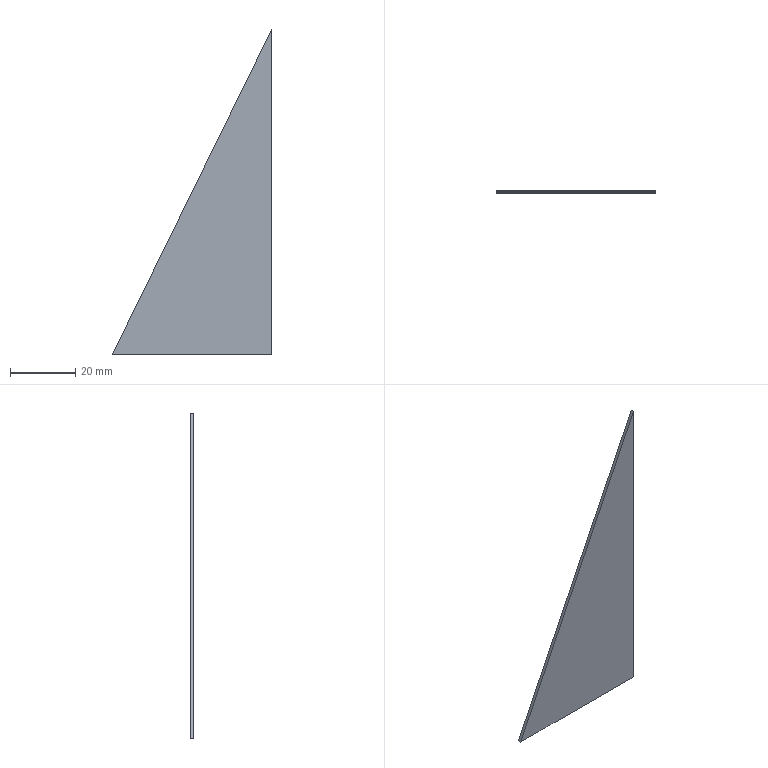Part | STEP file | RJWD-DY-0114_X2_75356C145B898_5 | 1 solid | 5 faces | box 48.998 x 1 x 99.996 mm | volume 2450 mm3 | plane 5
STEP:
#1=CARTESIAN_POINT('',(0.,0.,0.));
#2=DIRECTION('',(0.,0.,1.));
#3=DIRECTION('',(1.,0.,0.));
#4=AXIS2_PLACEMENT_3D('',#1,#2,#3);
#5=CARTESIAN_POINT('',(657.039,5199.7,119.644));
#6=VERTEX_POINT('',#5);
#7=CARTESIAN_POINT('',(657.039,5199.7,219.64));
#8=VERTEX_POINT('',#7);
#9=CARTESIAN_POINT('',(657.039,5199.7,119.644));
#10=DIRECTION('',(0.,0.,1.));
#11=VECTOR('',#10,1.);
#12=LINE('',#9,#11);
#13=CARTESIAN_POINT('',(608.041,5199.7,219.644));
#14=DIRECTION('',(0.,1.,0.));
#15=DIRECTION('',(0.,0.,1.));
#16=AXIS2_PLACEMENT_3D('',#13,#14,#15);
#17=PLANE('',#16);
#18=CARTESIAN_POINT('',(-100.,48.998));
#19=DIRECTION('',(1.,0.));
#20=VECTOR('',#19,1.);
#21=LINE('',#18,#20);
#22=(GEOMETRIC_REPRESENTATION_CONTEXT(2)PARAMETRIC_REPRESENTATION_CONTEXT()REPRESENTATION_CONTEXT('',''));
#23=DEFINITIONAL_REPRESENTATION('',(#21),#22);
#24=PCURVE('',#17,#23);
#25=CARTESIAN_POINT('',(657.039,5199.7,219.644));
#26=DIRECTION('',(-1.,0.,0.));
#27=DIRECTION('',(0.,0.,1.));
#28=AXIS2_PLACEMENT_3D('',#25,#26,#27);
#29=PLANE('',#28);
#30=CARTESIAN_POINT('',(-100.,0.));
#31=DIRECTION('',(1.,0.));
#32=VECTOR('',#31,1.);
#33=LINE('',#30,#32);
#34=(GEOMETRIC_REPRESENTATION_CONTEXT(2)PARAMETRIC_REPRESENTATION_CONTEXT()REPRESENTATION_CONTEXT('',''));
#35=DEFINITIONAL_REPRESENTATION('',(#33),#34);
#36=PCURVE('',#29,#35);
#37=SURFACE_CURVE('',#12,(#24,#36),.PCURVE_S1.);
#38=EDGE_CURVE('',#6,#8,#37,.T.);
#39=ORIENTED_EDGE('',*,*,#38,.F.);
#40=CARTESIAN_POINT('',(608.041,5199.7,119.644));
#41=VERTEX_POINT('',#40);
#42=CARTESIAN_POINT('',(657.039,5199.7,119.644));
#43=DIRECTION('',(-1.,0.,0.));
#44=VECTOR('',#43,1.);
#45=LINE('',#42,#44);
#46=CARTESIAN_POINT('',(-100.,48.998));
#47=DIRECTION('',(0.,-1.));
#48=VECTOR('',#47,1.);
#49=LINE('',#46,#48);
#50=(GEOMETRIC_REPRESENTATION_CONTEXT(2)PARAMETRIC_REPRESENTATION_CONTEXT()REPRESENTATION_CONTEXT('',''));
#51=DEFINITIONAL_REPRESENTATION('',(#49),#50);
#52=PCURVE('',#17,#51);
#53=CARTESIAN_POINT('',(0.,140.,119.644));
#54=DIRECTION('',(0.,0.,1.));
#55=DIRECTION('',(1.,0.,0.));
#56=AXIS2_PLACEMENT_3D('',#53,#54,#55);
#57=PLANE('',#56);
#58=CARTESIAN_POINT('',(657.039,5059.7));
#59=DIRECTION('',(-1.,0.));
#60=VECTOR('',#59,1.);
#61=LINE('',#58,#60);
#62=(GEOMETRIC_REPRESENTATION_CONTEXT(2)PARAMETRIC_REPRESENTATION_CONTEXT()REPRESENTATION_CONTEXT('',''));
#63=DEFINITIONAL_REPRESENTATION('',(#61),#62);
#64=PCURVE('',#57,#63);
#65=SURFACE_CURVE('',#45,(#52,#64),.PCURVE_S1.);
#66=EDGE_CURVE('',#6,#41,#65,.T.);
#67=ORIENTED_EDGE('',*,*,#66,.T.);
#68=CARTESIAN_POINT('',(657.039,5199.7,219.64));
#69=DIRECTION('',(-0.44,0.,-0.898));
#70=VECTOR('',#69,1.);
#71=LINE('',#68,#70);
#72=CARTESIAN_POINT('',(-0.004082,48.998));
#73=DIRECTION('',(-0.898,-0.44));
#74=VECTOR('',#73,1.);
#75=LINE('',#72,#74);
#76=(GEOMETRIC_REPRESENTATION_CONTEXT(2)PARAMETRIC_REPRESENTATION_CONTEXT()REPRESENTATION_CONTEXT('',''));
#77=DEFINITIONAL_REPRESENTATION('',(#75),#76);
#78=PCURVE('',#17,#77);
#79=CARTESIAN_POINT('',(657.041,140.,219.644));
#80=DIRECTION('',(-0.898,0.,0.44));
#81=DIRECTION('',(0.,1.,0.));
#82=AXIS2_PLACEMENT_3D('',#79,#80,#81);
#83=PLANE('',#82);
#84=CARTESIAN_POINT('',(5059.7,0.004545));
#85=DIRECTION('',(0.,1.));
#86=VECTOR('',#85,1.);
#87=LINE('',#84,#86);
#88=(GEOMETRIC_REPRESENTATION_CONTEXT(2)PARAMETRIC_REPRESENTATION_CONTEXT()REPRESENTATION_CONTEXT('',''));
#89=DEFINITIONAL_REPRESENTATION('',(#87),#88);
#90=PCURVE('',#83,#89);
#91=SURFACE_CURVE('',#71,(#78,#90),.PCURVE_S1.);
#92=EDGE_CURVE('',#8,#41,#91,.T.);
#93=ORIENTED_EDGE('',*,*,#92,.F.);
#94=EDGE_LOOP('',(#39,#67,#93));
#95=FACE_BOUND('',#94,.F.);
#96=ADVANCED_FACE('',(#95),#17,.F.);
#97=CARTESIAN_POINT('',(657.039,5200.7,119.644));
#98=VERTEX_POINT('',#97);
#99=CARTESIAN_POINT('',(657.039,5200.7,219.64));
#100=VERTEX_POINT('',#99);
#101=CARTESIAN_POINT('',(657.039,5200.7,119.644));
#102=DIRECTION('',(0.,0.,1.));
#103=VECTOR('',#102,1.);
#104=LINE('',#101,#103);
#105=CARTESIAN_POINT('',(-100.,1.));
#106=DIRECTION('',(1.,0.));
#107=VECTOR('',#106,1.);
#108=LINE('',#105,#107);
#109=(GEOMETRIC_REPRESENTATION_CONTEXT(2)PARAMETRIC_REPRESENTATION_CONTEXT()REPRESENTATION_CONTEXT('',''));
#110=DEFINITIONAL_REPRESENTATION('',(#108),#109);
#111=PCURVE('',#29,#110);
#112=CARTESIAN_POINT('',(657.039,5200.7,219.644));
#113=DIRECTION('',(0.,-1.,0.));
#114=DIRECTION('',(0.,0.,-1.));
#115=AXIS2_PLACEMENT_3D('',#112,#113,#114);
#116=PLANE('',#115);
#117=CARTESIAN_POINT('',(100.,0.));
#118=DIRECTION('',(-1.,0.));
#119=VECTOR('',#118,1.);
#120=LINE('',#117,#119);
#121=(GEOMETRIC_REPRESENTATION_CONTEXT(2)PARAMETRIC_REPRESENTATION_CONTEXT()REPRESENTATION_CONTEXT('',''));
#122=DEFINITIONAL_REPRESENTATION('',(#120),#121);
#123=PCURVE('',#116,#122);
#124=SURFACE_CURVE('',#104,(#111,#123),.PCURVE_S1.);
#125=EDGE_CURVE('',#98,#100,#124,.T.);
#126=ORIENTED_EDGE('',*,*,#125,.F.);
#127=CARTESIAN_POINT('',(657.039,5200.7,119.644));
#128=DIRECTION('',(0.,-1.,0.));
#129=VECTOR('',#128,1.);
#130=LINE('',#127,#129);
#131=CARTESIAN_POINT('',(-100.,1.));
#132=DIRECTION('',(0.,-1.));
#133=VECTOR('',#132,1.);
#134=LINE('',#131,#133);
#135=(GEOMETRIC_REPRESENTATION_CONTEXT(2)PARAMETRIC_REPRESENTATION_CONTEXT()REPRESENTATION_CONTEXT('',''));
#136=DEFINITIONAL_REPRESENTATION('',(#134),#135);
#137=PCURVE('',#29,#136);
#138=CARTESIAN_POINT('',(657.039,5060.7));
#139=DIRECTION('',(0.,-1.));
#140=VECTOR('',#139,1.);
#141=LINE('',#138,#140);
#142=(GEOMETRIC_REPRESENTATION_CONTEXT(2)PARAMETRIC_REPRESENTATION_CONTEXT()REPRESENTATION_CONTEXT('',''));
#143=DEFINITIONAL_REPRESENTATION('',(#141),#142);
#144=PCURVE('',#57,#143);
#145=SURFACE_CURVE('',#130,(#137,#144),.PCURVE_S1.);
#146=EDGE_CURVE('',#98,#6,#145,.T.);
#147=ORIENTED_EDGE('',*,*,#146,.T.);
#148=ORIENTED_EDGE('',*,*,#38,.T.);
#149=CARTESIAN_POINT('',(657.039,5199.7,219.64));
#150=DIRECTION('',(0.,1.,0.));
#151=VECTOR('',#150,1.);
#152=LINE('',#149,#151);
#153=CARTESIAN_POINT('',(-0.004082,0.));
#154=DIRECTION('',(0.,1.));
#155=VECTOR('',#154,1.);
#156=LINE('',#153,#155);
#157=(GEOMETRIC_REPRESENTATION_CONTEXT(2)PARAMETRIC_REPRESENTATION_CONTEXT()REPRESENTATION_CONTEXT('',''));
#158=DEFINITIONAL_REPRESENTATION('',(#156),#157);
#159=PCURVE('',#29,#158);
#160=CARTESIAN_POINT('',(5059.7,0.004545));
#161=DIRECTION('',(1.,0.));
#162=VECTOR('',#161,1.);
#163=LINE('',#160,#162);
#164=(GEOMETRIC_REPRESENTATION_CONTEXT(2)PARAMETRIC_REPRESENTATION_CONTEXT()REPRESENTATION_CONTEXT('',''));
#165=DEFINITIONAL_REPRESENTATION('',(#163),#164);
#166=PCURVE('',#83,#165);
#167=SURFACE_CURVE('',#152,(#159,#166),.PCURVE_S1.);
#168=EDGE_CURVE('',#8,#100,#167,.T.);
#169=ORIENTED_EDGE('',*,*,#168,.T.);
#170=EDGE_LOOP('',(#126,#147,#148,#169));
#171=FACE_BOUND('',#170,.F.);
#172=ADVANCED_FACE('',(#171),#29,.F.);
#173=CARTESIAN_POINT('',(608.041,5200.7,119.644));
#174=VERTEX_POINT('',#173);
#175=CARTESIAN_POINT('',(608.041,5200.7,119.644));
#176=DIRECTION('',(1.,0.,0.));
#177=VECTOR('',#176,1.);
#178=LINE('',#175,#177);
#179=CARTESIAN_POINT('',(100.,-48.998));
#180=DIRECTION('',(0.,1.));
#181=VECTOR('',#180,1.);
#182=LINE('',#179,#181);
#183=(GEOMETRIC_REPRESENTATION_CONTEXT(2)PARAMETRIC_REPRESENTATION_CONTEXT()REPRESENTATION_CONTEXT('',''));
#184=DEFINITIONAL_REPRESENTATION('',(#182),#183);
#185=PCURVE('',#116,#184);
#186=CARTESIAN_POINT('',(608.041,5060.7));
#187=DIRECTION('',(1.,0.));
#188=VECTOR('',#187,1.);
#189=LINE('',#186,#188);
#190=(GEOMETRIC_REPRESENTATION_CONTEXT(2)PARAMETRIC_REPRESENTATION_CONTEXT()REPRESENTATION_CONTEXT('',''));
#191=DEFINITIONAL_REPRESENTATION('',(#189),#190);
#192=PCURVE('',#57,#191);
#193=SURFACE_CURVE('',#178,(#185,#192),.PCURVE_S1.);
#194=EDGE_CURVE('',#174,#98,#193,.T.);
#195=ORIENTED_EDGE('',*,*,#194,.T.);
#196=ORIENTED_EDGE('',*,*,#125,.T.);
#197=CARTESIAN_POINT('',(608.041,5200.7,119.644));
#198=DIRECTION('',(0.44,0.,0.898));
#199=VECTOR('',#198,1.);
#200=LINE('',#197,#199);
#201=CARTESIAN_POINT('',(100.,-48.998));
#202=DIRECTION('',(-0.898,0.44));
#203=VECTOR('',#202,1.);
#204=LINE('',#201,#203);
#205=(GEOMETRIC_REPRESENTATION_CONTEXT(2)PARAMETRIC_REPRESENTATION_CONTEXT()REPRESENTATION_CONTEXT('',''));
#206=DEFINITIONAL_REPRESENTATION('',(#204),#205);
#207=PCURVE('',#116,#206);
#208=CARTESIAN_POINT('',(5060.7,111.36));
#209=DIRECTION('',(0.,-1.));
#210=VECTOR('',#209,1.);
#211=LINE('',#208,#210);
#212=(GEOMETRIC_REPRESENTATION_CONTEXT(2)PARAMETRIC_REPRESENTATION_CONTEXT()REPRESENTATION_CONTEXT('',''));
#213=DEFINITIONAL_REPRESENTATION('',(#211),#212);
#214=PCURVE('',#83,#213);
#215=SURFACE_CURVE('',#200,(#207,#214),.PCURVE_S1.);
#216=EDGE_CURVE('',#174,#100,#215,.T.);
#217=ORIENTED_EDGE('',*,*,#216,.F.);
#218=EDGE_LOOP('',(#195,#196,#217));
#219=FACE_BOUND('',#218,.F.);
#220=ADVANCED_FACE('',(#219),#116,.F.);
#221=CARTESIAN_POINT('',(608.041,5199.7,119.644));
#222=DIRECTION('',(0.,1.,0.));
#223=VECTOR('',#222,1.);
#224=LINE('',#221,#223);
#225=CARTESIAN_POINT('',(608.041,5059.7));
#226=DIRECTION('',(0.,1.));
#227=VECTOR('',#226,1.);
#228=LINE('',#225,#227);
#229=(GEOMETRIC_REPRESENTATION_CONTEXT(2)PARAMETRIC_REPRESENTATION_CONTEXT()REPRESENTATION_CONTEXT('',''));
#230=DEFINITIONAL_REPRESENTATION('',(#228),#229);
#231=PCURVE('',#57,#230);
#232=CARTESIAN_POINT('',(5059.7,111.36));
#233=DIRECTION('',(1.,0.));
#234=VECTOR('',#233,1.);
#235=LINE('',#232,#234);
#236=(GEOMETRIC_REPRESENTATION_CONTEXT(2)PARAMETRIC_REPRESENTATION_CONTEXT()REPRESENTATION_CONTEXT('',''));
#237=DEFINITIONAL_REPRESENTATION('',(#235),#236);
#238=PCURVE('',#83,#237);
#239=SURFACE_CURVE('',#224,(#231,#238),.PCURVE_S1.);
#240=EDGE_CURVE('',#41,#174,#239,.T.);
#241=ORIENTED_EDGE('',*,*,#240,.F.);
#242=ORIENTED_EDGE('',*,*,#66,.F.);
#243=ORIENTED_EDGE('',*,*,#146,.F.);
#244=ORIENTED_EDGE('',*,*,#194,.F.);
#245=EDGE_LOOP('',(#241,#242,#243,#244));
#246=FACE_BOUND('',#245,.F.);
#247=ADVANCED_FACE('',(#246),#57,.F.);
#248=ORIENTED_EDGE('',*,*,#216,.T.);
#249=ORIENTED_EDGE('',*,*,#168,.F.);
#250=ORIENTED_EDGE('',*,*,#92,.T.);
#251=ORIENTED_EDGE('',*,*,#240,.T.);
#252=EDGE_LOOP('',(#248,#249,#250,#251));
#253=FACE_BOUND('',#252,.F.);
#254=ADVANCED_FACE('',(#253),#83,.T.);
#255=CLOSED_SHELL('',(#96,#172,#220,#247,#254));
#256=MANIFOLD_SOLID_BREP('',#255);
#257=(LENGTH_UNIT()NAMED_UNIT(*)SI_UNIT(.MILLI.,.METRE.));
#258=UNCERTAINTY_MEASURE_WITH_UNIT(LENGTH_MEASURE(0.0000001),#257,'','');
#259=(NAMED_UNIT(*)PLANE_ANGLE_UNIT()SI_UNIT($,.RADIAN.));
#260=(NAMED_UNIT(*)SI_UNIT($,.STERADIAN.)SOLID_ANGLE_UNIT());
#261=(GEOMETRIC_REPRESENTATION_CONTEXT(3)GLOBAL_UNCERTAINTY_ASSIGNED_CONTEXT((#258))GLOBAL_UNIT_ASSIGNED_CONTEXT((#257,#259,#260))REPRESENTATION_CONTEXT('',''));
#262=ADVANCED_BREP_SHAPE_REPRESENTATION('',(#4,#256),#261);